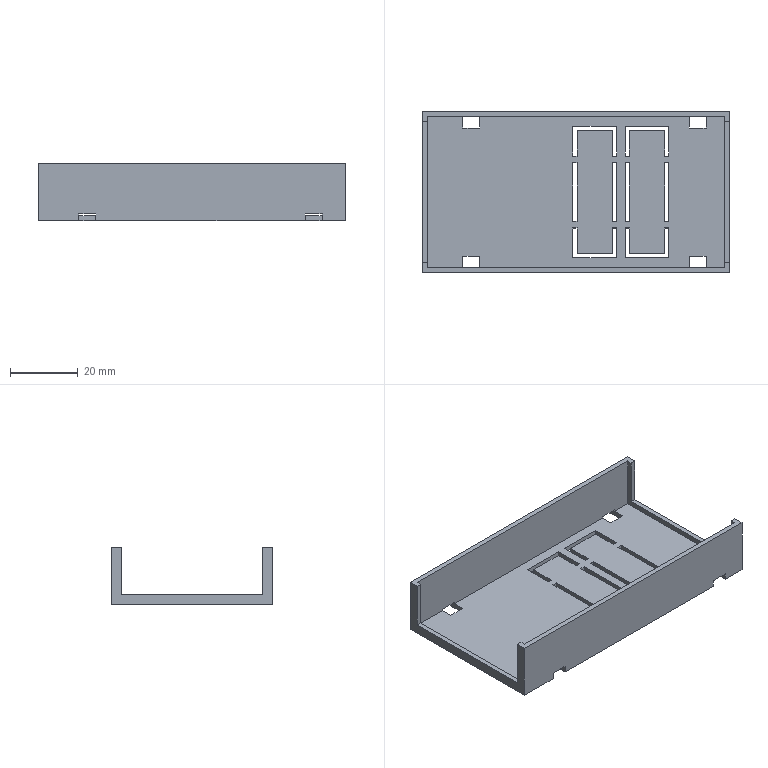Part | STEP file | K3HB_V_COVER. | 1 solid | 82 faces | box 91 x 47.87 x 17 mm | volume 10803 mm3 | plane 82